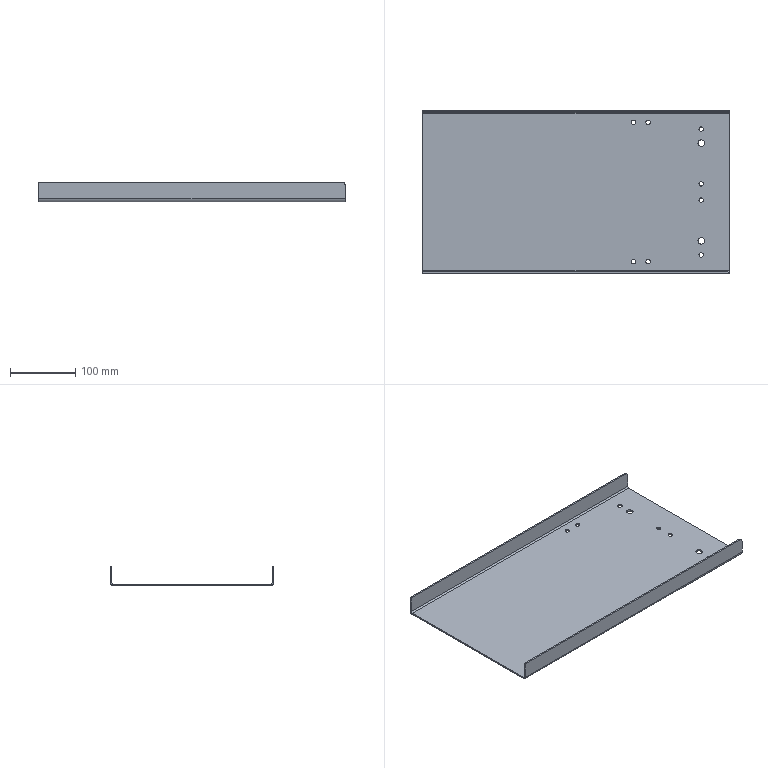Part | STEP file | [01]-9 | 1 solid | 36 faces | box 470 x 250 x 30 mm | volume 325882 mm3 | cylinder 26 | plane 10 | commonest cylinder face diameters 6.8 x16 10 x6 4.6 x2 9.2 x2